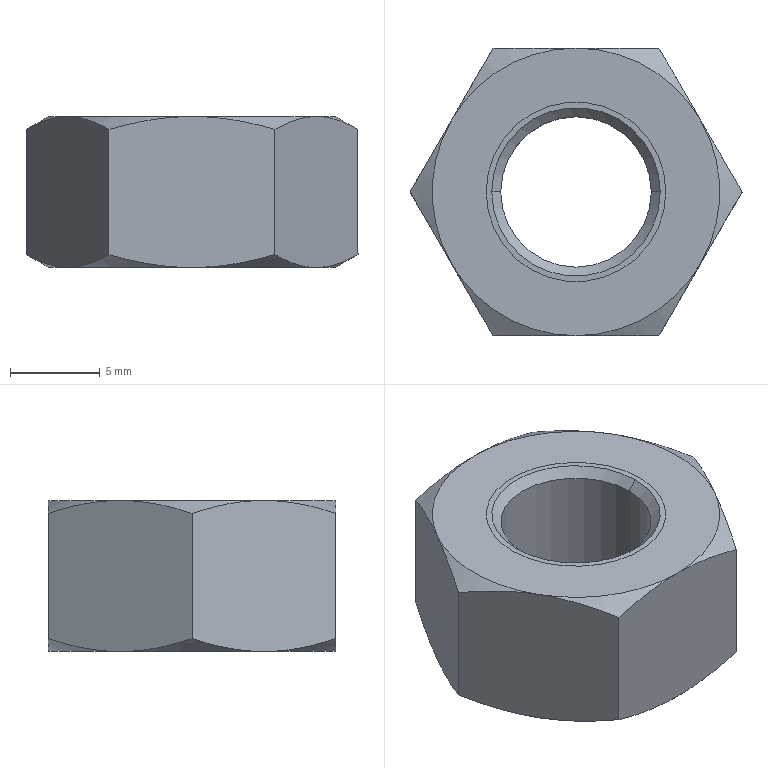Part | NX | features BREP 2 | 1 solid | 28 faces | box 18.475 x 16 x 8.4 mm | volume 1823 mm3 | cone 16 | plane 8 | cylinder 4 | commonest cylinder face diameters 8.376 x2 10 x2